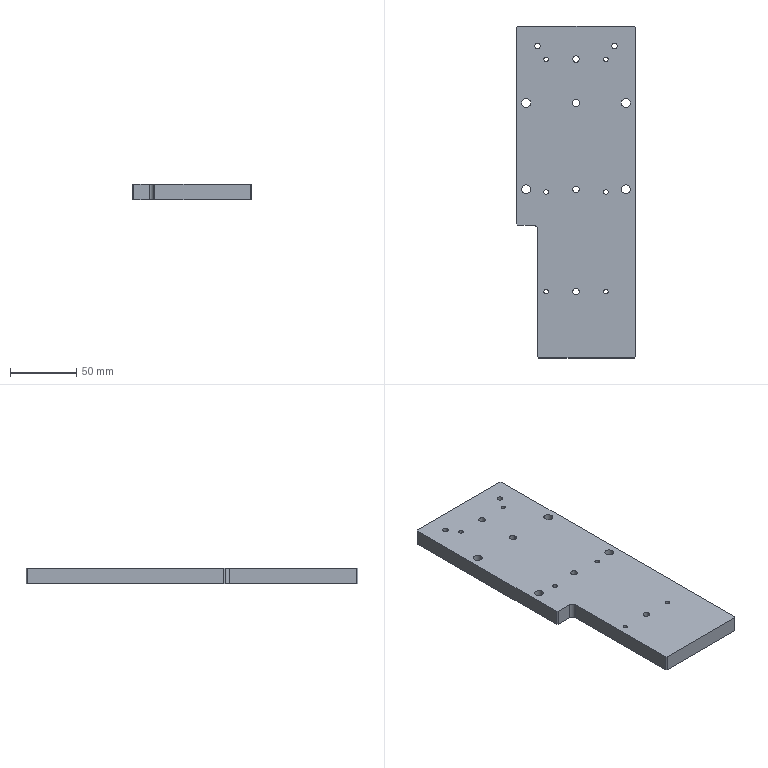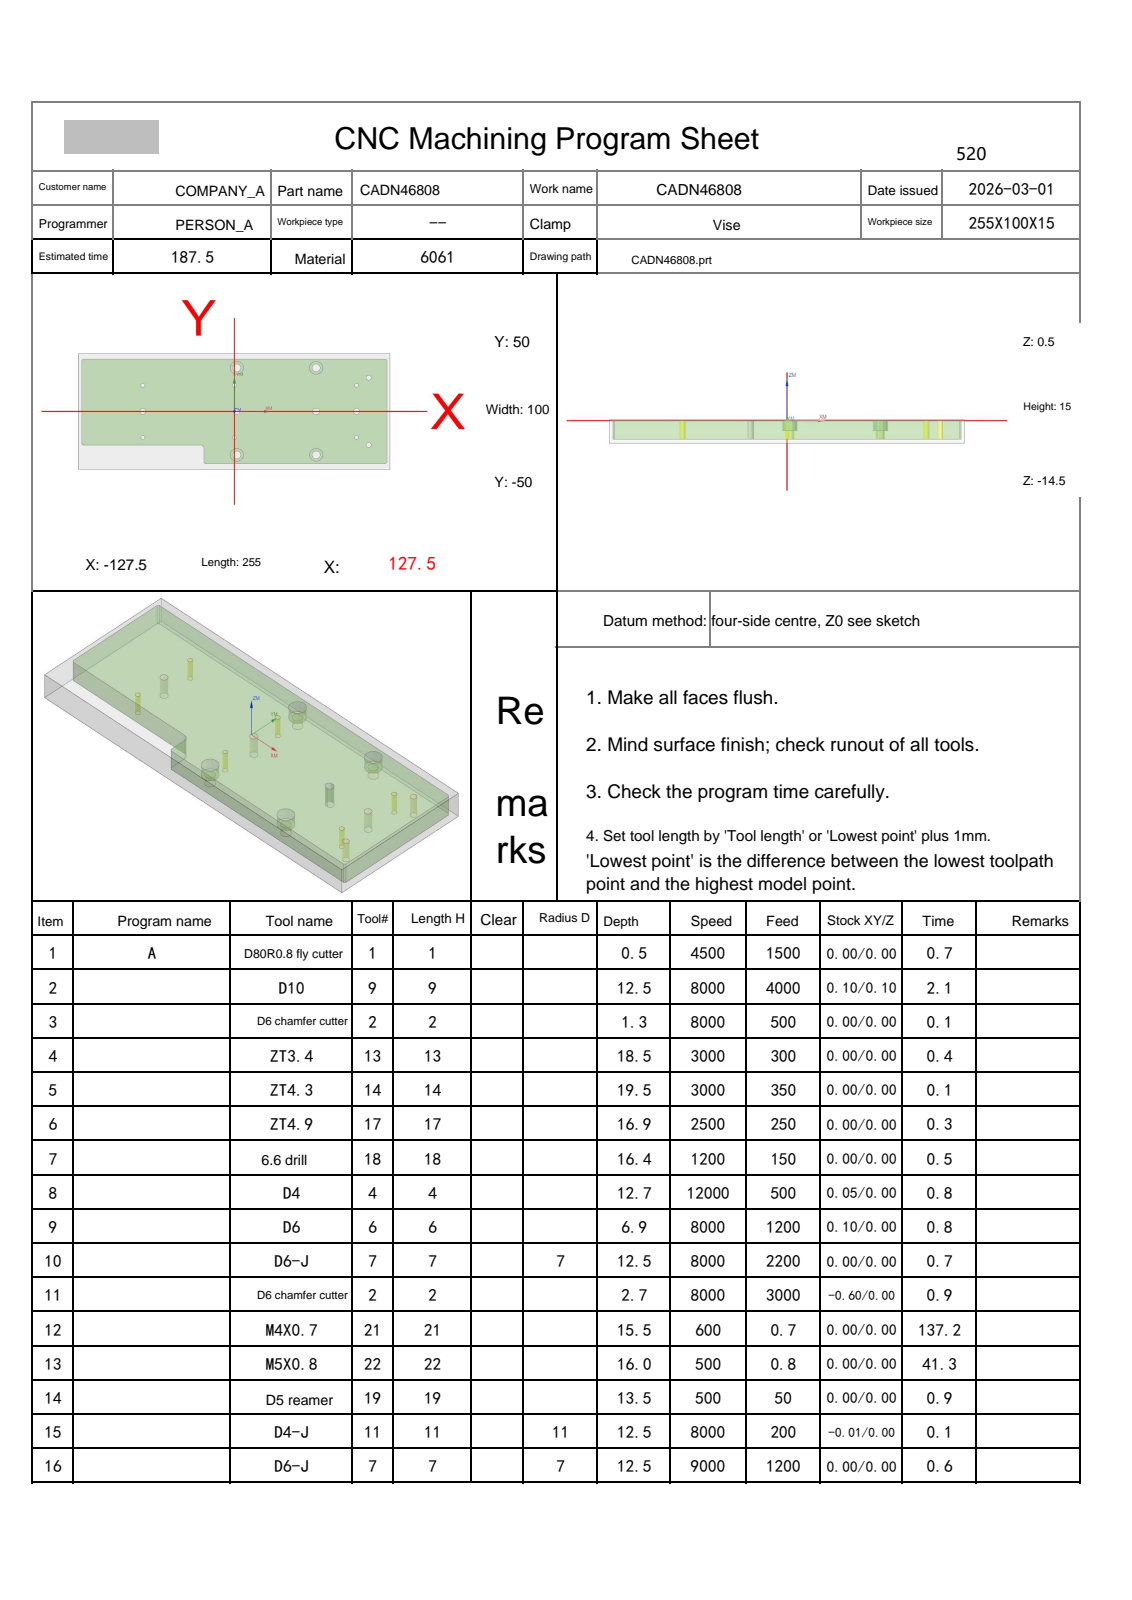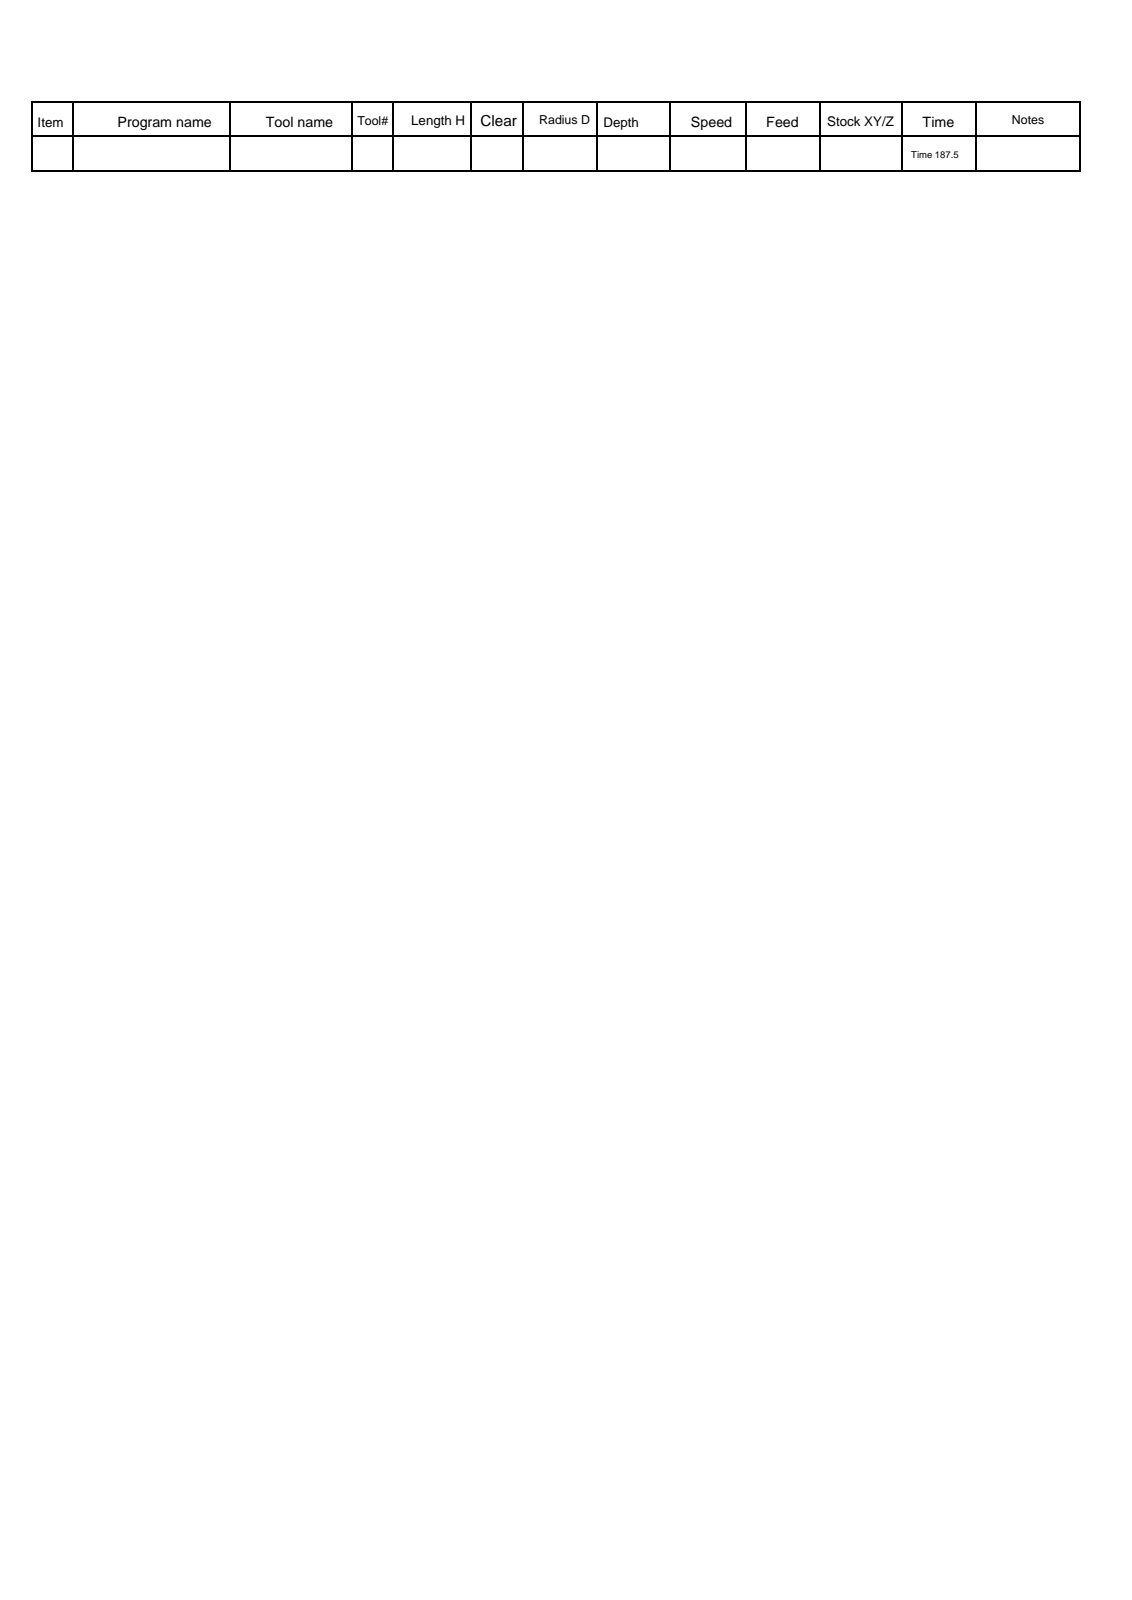NC program | NX | posted by the shop | part box 90 x 250 x 12 mm
Lines 1 to 1513 of 3445, first 1227 of 1511 lines:
%
O0001
(Machine time: 358.05 MIN)
(===Total Tool:14===)
(T1=D80R0.8 fly cutter D=80.  R=0.8  D-  H01 Z=0.    )
(T9=D10     D=10.  R=0.   D-  H09 Z=-12.  )
(T2=D6 chamfer cutter   D=6.   R=0.   D-  H02 Z=-2.2  )
(T13=ZT3.4  D=3.4  DR_a=118 D-  H13 Z=-18.  )
(T14=ZT4.3  D=4.3  DR_a=118 D-  H14 Z=-19.  )
(T17=ZT4.9  D=4.9  DR_a=120 D-  H17 Z=-16.41)
(T18=6.6 drill  D=6.6  DR_a=120 D-  H18 Z=-15.91)
(T4=D4      D=4.   R=0.   D-  H04 Z=-12.2 )
(T6=D6      D=6.   R=0.   D-  H06 Z=-6.4  )
(T7=D6-J    D=6.   R=0.   D7  H07 Z=-12.  )
(T21=M4X0.7 D=3.3  DR_a=180 D-  H21 Z=-15.  )
(T22=M5X0.8 D=4.2  DR_a=180 D-  H22 Z=-15.5 )
(T19=D5 reamer   D=5.   DR_a=180 D-  H19 Z=-13.  )
(T11=D4-J   D=4.   R=0.   D11 H11 Z=-12.  )
G80 G90 G17 G49 G40
G91 G28 Z0
M01
N1 T01 M06
(D80R0.8 fly cutter  D=80. R=0.8 H=01 ce=0.00 di=0.00)
G00 G90 G54 X-170. Y42.5 M03 S4500
G43 H01 Z50.
M08
Z2.
G01 Z0.0 F1500.
X-165.
X165.
Y0.0
X-165.
Y-42.5
X165.
X170.
Z2.
G00 Z50.
G91 G28 Z0.0
M05
M09
G91 G28 Z0.0
M01
N2 T09 M06
(D10  D=10. R=0. H=09 ce=0.10 di=0.10)
G00 G90 G54 X-125.158 Y61.447 M03 S8000
G43 H09 Z50.
M08
Z-10.
G01 X-125.141 Y61.348 Z-10.625 F4000.
X-125.125 Y61.25 Z-10.872
X-125.109 Y61.151 Z-11.054
X-125.092 Y61.052 Z-11.2
X-125.076 Y60.954 Z-11.323
X-125.06 Y60.855 Z-11.428
X-125.043 Y60.756 Z-11.52
X-125.027 Y60.658 Z-11.6
X-125.011 Y60.559 Z-11.67
X-124.994 Y60.46 Z-11.732
X-124.978 Y60.362 Z-11.786
X-124.962 Y60.263 Z-11.833
X-124.945 Y60.164 Z-11.874
X-124.929 Y60.066 Z-11.908
X-124.913 Y59.967 Z-11.936
X-124.896 Y59.868 Z-11.96
X-124.88 Y59.77 Z-11.977
X-124.864 Y59.671 Z-11.99
X-124.847 Y59.573 Z-11.997
X-124.831 Y59.474 Z-12.
X-124.487 Y57.397
G03 X-124.17 Y57.008 I.503 J.086
X-120.255 Y56.356 I4.038 J12.171
X-111.283 Y56.191 I8.972 J243.457
X-109.151 Y56.2 I0.0 J243.623
G01 X125.648 Y56.182
G02 X132.353 Y51.481 I-.009 J-7.145
X133.525 Y45.381 I-18.068 J-6.633
X133.718 Y35.276 I-263.984 J-10.105
X133.699 Y32.104 I-264.177 J0.0
G01 X133.679 Y-48.196
G02 X129.116 Y-54.791 I-7.099 J.036
X123.108 Y-56.009 I-6.605 J17.156
X113.899 Y-56.213 I-9.209 J207.731
X111.431 Y-56.199 I0.0 J207.935
G01 X-125.589 Y-56.184
X-125.654 Y-56.185
G02 X-132.289 Y-51.621 I0.0 J7.105
X-133.519 Y-45.454 I17.459 J6.69
X-133.712 Y-36.317 I217.075 J9.137
X-133.699 Y-33.937 I217.267 J0.0
G01 X-133.675 Y48.283
G02 X-129.102 Y54.798 I7.095 J-.117
X-124.661 Y55.615 I4.441 J-11.659
X-124.243 Y55.608 I0.0 J-12.476
G03 X-107.231 Y55.401 I18.077 J785.537
G01 X123.788 Y55.382
G02 X130.819 Y50.947 I-.125 J-7.989
X132.545 Y44.658 I-15.2 J-7.553
X132.897 Y36.148 I-102.586 J-8.509
X132.89 Y34.908 I-102.938 J0.0
G01 X132.878 Y-46.347
G02 X128.402 Y-53.339 I-8.005 J.196
X122.108 Y-55.05 I-7.546 J15.331
X113.513 Y-55.399 I-8.594 J105.535
X112.198 Y-55.391 I0.0 J105.885
G01 X-123.847 Y-55.378
G02 X-130.812 Y-50.953 I.187 J7.987
X-132.534 Y-44.747 I15.044 J7.517
X-132.9 Y-36.07 I102.672 J8.678
X-132.891 Y-34.678 I103.038 J0.0
G01 X-132.878 Y46.347
G02 X-127.751 Y53.506 I7.741 J-.128
X-121.795 Y54.573 I6.129 J-17.049
X-113.953 Y54.638 I7.842 J-472.
X-108.11 Y54.602 I0.0 J-472.066
G01 X122.028 Y54.58
G02 X129.881 Y49.564 I-.191 J-8.954
X131.724 Y42.728 I-16.901 J-8.222
X132.097 Y33.636 I-110.49 J-9.092
X132.09 Y32.339 I-110.863 J0.0
G01 X132.075 Y-44.601
G02 X127.083 Y-52.368 I-8.949 J.264
X120.403 Y-54.203 I-8.157 J16.616
X111.152 Y-54.599 I-9.251 J107.876
X109.695 Y-54.589 I0.0 J108.272
G01 X-121.965 Y-54.581
G02 X-129.839 Y-49.637 I.129 J8.948
X-131.723 Y-42.73 I16.736 J8.274
X-132.099 Y-33.56 I111.633 J9.171
X-132.09 Y-32.181 I112.009 J0.0
G01 X-132.081 Y44.439
G02 X-126.86 Y52.213 I8.466 J-.046
X-120.33 Y53.637 I7.215 J-17.401
X-112.344 Y53.823 I7.986 J-171.457
X-109.789 Y53.804 I0.0 J-171.642
G01 X120.268 Y53.779
G02 X128.972 Y48.325 I-.054 J-9.759
X130.894 Y41.182 I-18.023 J-8.678
X131.285 Y32.798 I-89.73 J-8.384
X131.28 Y31.835 I-90.121 J0.0
G01 X131.276 Y-42.785
G02 X125.794 Y-51.483 I-9.715 J.047
X118.801 Y-53.379 I-8.62 J17.949
X108.985 Y-53.801 I-9.816 J114.068
X107.373 Y-53.789 I0.0 J114.489
G01 X-120.287 Y-53.776
G02 X-129.121 Y-48.018 I.09 J9.793
X-130.904 Y-41.081 I18.797 J8.529
X-131.294 Y-31.667 I113.427 J9.414
X-131.287 Y-30.452 I113.817 J0.0
G01 X-131.275 Y42.808
Y42.811
G02 X-126.128 Y50.963 I9.029 J0.0
X-119.506 Y52.693 I7.884 J-16.63
X-111.144 Y53.008 I8.362 J-110.839
X-109.595 Y52.998 I0.0 J-111.154
G01 X118.545 Y52.981
X118.682 Y52.982
G02 X125.84 Y50.186 I0.0 J-10.562
G01 X126.615 Y49.372
G02 X129.219 Y46.866 I-5.969 J-8.805
X130.1 Y44.011 I-4.262 J-2.88
G03 X130.338 Y37.709 I135.671 J1.964
G02 X130.511 Y23.708 I-564.408 J-14.002
X130.498 Y19.791 I-564.581 J0.0
G01 X130.476 Y-41.069
G02 X130.1 Y-44.015 I-15.522 J.487
X128.388 Y-47.893 I-5.645 J.175
X121.214 Y-51.9 I-10.145 J9.738
X112.565 Y-52.883 I-9.072 J41.292
X101.253 Y-53.001 I-11.313 J540.846
X99.287 Y-52.998 I0.0 J540.964
G01 X-118.613 Y-52.975
X-118.717 Y-52.976
G02 X-126.168 Y-49.851 I0.0 J10.446
X-129.498 Y-43.2 I10.497 J9.414
X-130.406 Y-34.301 I45.044 J9.093
X-130.503 Y-22.532 I709.373 J11.77
X-130.498 Y-19.742 I709.47 J0.0
G01 X-130.477 Y41.038
G02 X-130.1 Y44.015 I20.16 J-1.041
X-128.283 Y47.946 I5.53 J-.17
X-123.993 Y50.623 I7.387 J-7.061
X-116.302 Y52.001 I8.574 J-25.718
X-106.011 Y52.215 I10.291 J-247.077
X-103.266 Y52.2 I0.0 J-247.291
G01 X116.954 Y52.18
X117.046
G02 X123.911 Y50.124 I0.0 J-12.489
G01 X125.329 Y49.928
G02 X126.672 Y49.334 I-9.033 J-22.267
G03 X125.329 Y49.928 I-10.376 J-21.674
G02 X121.666 Y50.698 I1.686 J17.109
G03 X114.654 Y51.504 I-7.012 J-30.093
G01 X114.448
G03 X105.805 Y51.562 I-8.644 J-639.404
X104.209 Y51.56 I0.0 J-639.462
G01 X-109.851 Y51.536
G03 X-110.63 Y51.541 I-.779 J-68.539
X-119.426 Y50.974 I0.0 J-68.544
X-123.087 Y50.1 I4.092 J-25.239
X-123.63 Y50.12 I-.542 J-7.145
X-125.563 Y49.854 I0.0 J-7.166
G01 X-126.66 Y49.351
X-125.563 Y49.854
X-124.821 Y50.034
G02 X-123.493 Y50.106 I1.328 J-12.134
X-123.087 Y50.1 I0.0 J-12.206
G03 X-117.888 Y50.386 I-.022 J47.735
G02 X-105.511 Y50.769 I12.377 J-199.641
X-103.177 Y50.756 I0.0 J-200.024
G01 X111.523 Y50.737
G02 X112.333 Y50.744 I.809 J-46.827
X119.652 Y50.169 I0.0 J-46.834
G01 X120.018 Y50.1
X123.998
X-124.061
G03 X-127.621 Y48.592 I.204 J-5.438
X-129.2 Y46.893 I9.138 J-10.075
X-130.1 Y43.923 I4.451 J-2.97
G01 Y43.906
Y-28.038
G02 X-129.702 Y-35.726 I-147.609 J-11.494
G03 X-128.536 Y-43.781 I33.867 J.789
X-124.572 Y-49.841 I11.22 J3.013
X-118.695 Y-52.007 I6.982 J9.888
X-111.231 Y-52.363 I7.464 J77.978
X-109.827 Y-52.351 I0.0 J78.335
G01 X107.273 Y-52.335
G03 X108.249 Y-52.341 I.977 J83.987
X117.971 Y-51.776 I0.0 J83.993
X123.877 Y-50.107 I-2.72 J20.908
X127.621 Y-48.592 I-.033 J5.464
X129.2 Y-46.892 I-11.663 J12.422
G02 X127.621 Y-48.592 I-10.674 J8.336
X123.793 Y-50.122 I-3.828 J4.021
X123.43 Y-50.11 I0.0 J5.552
G01 X117.478 Y-50.983
G02 X106.712 Y-51.537 I-10.766 J104.313
X105.897 Y-51.534 I0.0 J104.867
G01 X-111.443
G02 X-112.157 Y-51.54 I-.714 J44.451
X-118.698 Y-51.056 I0.0 J44.456
X-126.998 Y-44.388 I1.814 J10.756
X-128.698 Y-37.01 I22.356 J9.038
X-129.095 Y-31.098 I548.53 J39.845
G01 X-129.496 Y-30.406
G02 X-130.076 Y-28.23 I4.84 J2.454
G03 X-129.096 Y-31.038 I5.199 J.239
G02 X-128.366 Y-34.531 I-12.801 J-4.499
G03 X-127.217 Y-41.366 I44.929 J4.034
X-123.445 Y-47.662 I12.084 J2.963
X-117.035 Y-50.379 I8.114 J10.225
X-109.247 Y-50.901 I7.788 J57.793
X-108.419 Y-50.895 I0.0 J58.316
G01 X105.401 Y-50.892
G03 X106.334 Y-50.897 I.932 J104.039
X117.379 Y-50.309 I0.0 J104.043
G01 X118.951 Y-50.1
X123.671
X-107.582 Y-50.097
G02 X-108.465 Y-50.103 I-.883 J57.401
X-116.118 Y-49.591 I0.0 J57.408
X-122.714 Y-46.577 I1.589 J12.202
X-126.399 Y-40.111 I9.76 J9.845
X-127.68 Y-33.679 I70.118 J17.316
G03 X-128.14 Y-32.072 I-5.489 J-.701
G01 X-129.096 Y-31.038
G02 X-127.918 Y-32.359 I-27.507 J-25.723
X-126.792 Y-35.753 I-11.626 J-5.739
G03 X-124.972 Y-41.778 I30.45 J5.914
X-116.844 Y-48.473 I10.835 J4.873
X-109.315 Y-49.379 I7.791 J32.981
X-98.956 Y-49.479 I10.359 J540.85
X-97.316 Y-49.476 I0.0 J540.949
G01 X-26.456
X-25.32 Y-49.926
X-24.002 Y-50.1
X-25.32 Y-49.926
G03 X-29.695 Y-48.872 I-4.651 J-9.695
X-38.394 Y-48.664 I-8.699 J-182.449
X-40.57 Y-48.677 I0.0 J-182.657
G01 X-104.948 Y-48.654
G02 X-105.805 Y-48.66 I-.856 J61.413
X-114.043 Y-48.105 I0.0 J61.419
X-120.626 Y-45.369 I1.815 J13.655
X-124.817 Y-39.084 I9.226 J10.691
G01 X-126.476 Y-34.003
G03 X-126.899 Y-33.149 I-3.394 J-1.148
G02 X-128.116 Y-32.096 I4.596 J6.545
G03 X-126.775 Y-33.25 I6.473 J6.166
G02 X-125.391 Y-35.831 I-6.932 J-5.38
G03 X-123.052 Y-41.105 I32.848 J11.413
X-115.195 Y-46.923 I10.924 J6.539
X-107.435 Y-47.919 I8.207 J33.22
X-97.449 Y-48.038 I9.987 J418.237
X-95.997 Y-48.035 I0.0 J418.356
G01 X-35.499 Y-48.061
G02 X-34.723 Y-48.055 I.777 J-48.885
X-28.37 Y-48.469 I0.0 J-48.891
X-27.493 Y-48.693 I-1.559 J-7.951
G01 X-26.55 Y-49.417
G03 X-28.455 Y-48.183 I-4.66 J-5.107
X-33.158 Y-47.424 I-5.177 J-17.137
X-43.01 Y-47.223 I-9.852 J-241.104
X-45.528 Y-47.236 I0.0 J-241.306
G01 X-102.708 Y-47.21
G02 X-103.459 Y-47.214 I-.751 J64.868
X-112.042 Y-46.644 I0.0 J64.872
X-119.146 Y-43.739 I1.918 J14.829
X-123.329 Y-38.198 I10.308 J12.129
G03 X-125.375 Y-34.186 I-39.67 J-17.707
X-125.778 Y-33.736 I-1.507 J-.946
G02 X-126.867 Y-33.173 I.914 J3.103
G03 X-125.633 Y-33.804 I2.442 J3.255
G02 X-123.924 Y-35.976 I-4.861 J-5.585
G03 X-120.932 Y-40.698 I33.01 J17.605
X-112.702 Y-45.637 I11.094 J9.161
X-104.041 Y-46.516 I8.742 J42.995
X-94.093 Y-46.595 I9.948 J627.526
G01 X-93.642
X-39.179 Y-46.622
G02 X-38.433 Y-46.617 I.746 J-61.427
X-30.881 Y-47.083 I0.0 J-61.431
X-28.36 Y-47.81 I-.809 J-7.548
G01 X-27.608 Y-48.605
G03 X-29.105 Y-47.257 I-4.624 J-3.631
X-33.248 Y-46.194 I-5.094 J-11.257
X-42.27 Y-45.797 I-9.022 J-102.322
X-43.625 Y-45.806 I0.0 J-102.719
G01 X-100.848 Y-45.764
G02 X-101.511 Y-45.768 I-.662 J64.43
X-110.419 Y-45.149 I0.0 J64.433
X-118.072 Y-41.919 I2.152 J15.777
X-122.182 Y-37.079 I14.004 J16.059
G03 X-124.537 Y-34.083 I-12.61 J-7.489
X-125.32 Y-33.926 I-.864 J-2.273
G01 X-125.763 Y-33.743
G03 X-124.569 Y-34.036 I1.357 J2.946
G02 X-122.429 Y-35.965 I-3.339 J-5.856
G03 X-118.715 Y-40.263 I32.322 J24.17
X-110.256 Y-44.341 I11.188 J12.397
X-101.075 Y-45.101 I9.182 J55.048
G01 X-100.859
X-91.179 Y-45.155
X-42.531 Y-45.177
G02 X-41.583 Y-45.171 I.948 J-75.978
X-32.992 Y-45.658 I0.0 J-75.984
X-29.319 Y-46.724 I-1.044 J-10.457
G03 X-28.462 Y-47.702 I7.628 J5.83
G02 X-29.438 Y-46.558 I6.867 J6.85
G03 X-32.505 Y-45.208 I-4.287 J-5.578
X-39.978 Y-44.458 I-7.709 J-39.258
X-51.174 Y-44.355 I-11.196 J-608.546
G01 X-51.929 Y-44.356
X-98.528 Y-44.326
G02 X-99.284 Y-44.33 I-.755 J70.472
X-108.66 Y-43.703 I0.0 J70.476
X-119.757 Y-37.686 I2.384 J17.638
G03 X-122.897 Y-34.49 I-22.64 J-19.098
X-123.836 Y-34.089 I-.94 J-.9
G01 X-124.002 Y-34.1
X-124.715 Y-34.006
G03 X-123.434 Y-34.109 I1.475 J10.344
G02 X-121.044 Y-35.669 I-2.29 J-6.116
G03 X-116.773 Y-39.483 I38.096 J38.367
X-107.791 Y-43.043 I11.559 J16.054
X-98.159 Y-43.683 I9.632 J72.154
X-97.58 Y-43.68 I0.0 J72.794
G01 X-87.34 Y-43.716
X-45.01 Y-43.737
G02 X-44.05 Y-43.731 I.961 J-85.296
X-34.803 Y-44.234 I0.0 J-85.302
X-30.319 Y-45.509 I-1.31 J-13.134
X-29.657 Y-46.079 I-.498 J-1.247
G01 X-29.256 Y-46.772
G03 X-29.946 Y-45.604 I-7.483 J-3.637
X-32.968 Y-44.04 I-4.549 J-5.085
X-40.283 Y-43.085 I-7.957 J-32.453
X-51.884 Y-42.904 I-11.601 J-371.949
X-54.806 Y-42.915 I0.0 J-372.13
G01 X-96.466 Y-42.886
G02 X-97.185 Y-42.89 I-.718 J77.858
X-106.841 Y-42.289 I0.0 J77.861
X-118.206 Y-37.029 I2.733 J20.814
G03 X-121.705 Y-34.32 I-17.187 J-18.584
G01 X-122.221 Y-34.1
X-123.581
G02 X-122.961 Y-34.078 I.62 J-8.938
X-121.854 Y-34.147 I0.0 J-8.96
X-118.866 Y-35.839 I-3.316 J-9.337
G03 X-113.29 Y-39.494 I22.228 J27.832
X-104.202 Y-41.861 I11.073 J23.891
X-93.972 Y-42.271 I10.231 J127.253
X-92.694 Y-42.265 I0.0 J127.664
G01 X-46.853 Y-42.299
G02 X-45.959 Y-42.295 I.895 J-88.655
X-36.167 Y-42.837 I0.0 J-88.659
X-31.107 Y-44.288 I-1.505 J-14.794
X-29.925 Y-45.257 I-1.351 J-2.854
G01 X-29.677 Y-46.017
G03 X-30.293 Y-44.634 I-3.43 J-.699
X-33.557 Y-42.803 I-5.064 J-5.203
X-41.197 Y-41.687 I-8.499 J-31.485
X-52.375 Y-41.469 I-11.178 J-286.059
X-54.329 Y-41.475 I0.0 J-286.278
G01 X-94.688 Y-41.445
G02 X-95.452 Y-41.449 I-.764 J80.238
X-105.621 Y-40.802 I0.0 J80.242
X-116.731 Y-36.282 I3.712 J25.037
G03 X-120.35 Y-34.119 I-13.265 J-18.091
G01 X-122.212 Y-34.1
G02 X-121.831 Y-34.098 I.381 J-44.546
X-120.085 Y-34.132 I0.0 J-44.548
X-116.915 Y-35.559 I-3.127 J-11.182
G03 X-110.243 Y-38.87 I19.711 J31.34
X-100.745 Y-40.578 I10.996 J33.882
X-89.198 Y-40.848 I11.547 J246.81
X-86.509 Y-40.833 I0.0 J247.08
G01 X-49.089 Y-40.857
G02 X-48.105 Y-40.852 I.985 J-100.333
X-37.656 Y-41.397 I0.0 J-100.338
X-31.869 Y-42.982 I-1.649 J-17.375
X-30.069 Y-44.492 I-1.934 J-4.135
G01 X-29.963 Y-45.139
G03 X-31.064 Y-43.107 I-2.563 J-.074
X-35.671 Y-41.107 I-6.662 J-9.037
X-44.631 Y-40.167 I-9.525 J-47.665
X-56.596 Y-40.031 I-11.965 J-524.426
X-58.649 Y-40.035 I0.0 J-524.562
G01 X-92.708 Y-40.007
G02 X-93.537 Y-40.011 I-.829 J88.735
X-104.123 Y-39.377 I0.0 J88.739
X-115.045 Y-35.621 I4.412 J30.583
G03 X-118.243 Y-34.1 I-11.321 J-19.686
G01 X-120.403
G02 X-119.45 Y-34.078 I.953 J-20.374
X-117.651 Y-34.157 I0.0 J-20.396
X-114.579 Y-35.28 I-4.054 J-15.855
G03 X-105.622 Y-38.369 I16.997 J34.749
X-94.877 Y-39.316 I10.937 J62.686
X-84.096 Y-39.399 I10.782 J698.601
X-81.598 Y-39.395 I0.0 J698.684
G01 X-50.137 Y-39.423
G02 X-49.422 Y-39.421 I.715 J-99.596
X-38.627 Y-40.007 I0.0 J-99.599
X-32.54 Y-41.658 I-1.983 J-19.367
X-30.137 Y-43.697 I-2.224 J-5.055
G01 X-30.041 Y-44.556
Y-44.539
G03 X-30.222 Y-43.34 I-4.075 J0.0
X-32.707 Y-41.062 I-4.758 J-2.696
X-39.038 Y-39.267 I-8.418 J-17.636
X-49.907 Y-38.636 I-10.869 J-93.311
G01 X-50.219 Y-38.637
X-60.408 Y-38.595
X-91.568 Y-38.561
G02 X-92.197 Y-38.564 I-.628 J90.084
X-103.141 Y-37.896 I0.0 J90.087
X-113.216 Y-34.955 I5.947 J39.101
G03 X-115.484 Y-34.1 I-29.245 J-74.121
G01 X-118.124
G02 X-116.943 Y-34.082 I1.181 J-39.028
X-114.819 Y-34.14 I0.0 J-39.046
X-110.467 Y-35.393 I-6.293 J-30.034
G03 X-96.796 Y-37.759 I14.988 J45.929
X-83.318 Y-37.973 I13.478 J424.552
X-79.358 Y-37.954 I0.0 J424.766
G01 X-51.342 Y-37.988
G02 X-50.754 Y-37.986 I.588 J-100.964
X-39.516 Y-38.613 I0.0 J-100.966
X-32.946 Y-40.415 I-2.194 J-20.879
X-30.18 Y-42.81 I-2.55 J-5.739
X-30.08 Y-43.534 I-2.558 J-.724
X-30.1 Y-43.862 I-2.659 J0.0
G03 X-30.076 Y-43.469 I-3.203 J.393
X-30.274 Y-42.357 I-3.227 J0.0
X-32.94 Y-39.878 I-5.312 J-3.04
X-39.611 Y-37.908 I-9.016 J-18.254
X-50.919 Y-37.207 I-11.308 J-90.848
G01 X-51.029
X-61.848 Y-37.155
X-89.588 Y-37.125
G02 X-90.363 Y-37.128 I-.775 J101.669
X-101.963 Y-36.465 I0.0 J101.672
X-111.57 Y-34.178 I8.745 J58.075
G01 X-111.883 Y-34.1
X-115.323
G02 X-113.678 Y-34.077 I1.645 J-59.152
X-110.703 Y-34.152 I0.0 J-59.175
X-104.836 Y-35.305 I-24.317 J-139.213
G03 X-91.701 Y-36.441 I13.343 J77.751
X-80.947 Y-36.521 I10.754 J728.148
X-77.941 Y-36.514 I0.0 J728.227
G01 X-53.178 Y-36.544
G02 X-52.491 Y-36.542 I.686 J-111.331
X-40.617 Y-37.177 I0.0 J-111.333
X-33.529 Y-39.042 I-2.405 J-23.54
X-30.339 Y-41.612 I-2.992 J-6.978
X-30.1 Y-42.143 I-2.84 J-1.599
G01 Y-43.023
G03 X-30.076 Y-42.598 I-3.798 J.424
X-30.252 Y-41.453 I-3.822 J0.0
X-32.915 Y-38.804 I-5.538 J-2.905
X-39.481 Y-36.653 I-9.347 J-17.434
X-50.658 Y-35.801 I-11.564 J-77.938
G01 X-60.409 Y-35.715
X-88.788 Y-35.678
G02 X-89.35 Y-35.68 I-.562 J102.536
X-102.432 Y-34.842 I0.0 J102.537
G01 X-106.585 Y-34.1
X-111.385
G02 X-108.711 Y-34.076 I2.674 J-150.193
X-103.902 Y-34.153 I0.0 J-150.217
G03 X-86.468 Y-35.061 I17.435 J166.899
X-85.469 Y-35.058 I0.0 J167.808
G01 X-54.142 Y-35.109
G02 X-53.546 Y-35.108 I.596 J-110.469
X-41.196 Y-35.8 I0.0 J-110.471
X-33.717 Y-37.83 I-2.619 J-24.445
X-30.334 Y-40.624 I-3.236 J-7.364
X-30.1 Y-41.168 I-2.458 J-1.38
G01 Y-42.128
G03 X-30.08 Y-41.67 I-5.337 J.458
X-30.18 Y-40.639 I-5.357 J0.0
X-32.492 Y-37.967 I-5.287 J-2.237
X-38.926 Y-35.492 I-9.576 J-15.297
X-49.515 Y-34.432 I-11.662 J-63.044
X-63.758 Y-34.264 I-14.243 J-605.708
X-67.369 Y-34.275 I0.0 J-605.876
G01 X-88.049 Y-34.23
G03 X-100.22 Y-34.077 I-12.171 J-482.238
X-104.96 Y-34.1 I0.0 J-482.392
G01 X-45.452 Y-34.12
G02 X-35.5 Y-35.901 I-.871 J-33.565
X-30.86 Y-38.844 I-3.536 J-10.705
X-30.1 Y-40.12 I-2.641 J-2.437
G01 Y-41.08
G03 X-30.075 Y-40.611 I-4.413 J.469
X-30.239 Y-39.416 I-4.438 J0.0
X-32.882 Y-36.578 I-5.911 J-2.856
X-39.593 Y-34.1 I-10.061 J-16.919
G01 X-46.153
X-38.326 Y-34.123
G02 X-31.145 Y-37.435 I-1.233 J-12.117
X-30.1 Y-39.044 I-2.856 J-2.997
G01 Y-40.004
G03 X-30.077 Y-39.54 I-4.601 J.464
X-30.234 Y-38.343 I-4.625 J0.0
X-32.891 Y-35.45 I-5.951 J-2.799
X-35.786 Y-34.1 I-6.516 J-10.194
G01 X-38.746
G02 X-37.44 Y-34.079 I1.305 J-39.724
X-35.147 Y-34.145 I0.0 J-39.745
X-30.269 Y-37.534 I-1.436 J-7.27
G01 X-30.1 Y-37.972
Y-38.932
G03 X-30.076 Y-38.463 I-4.52 J.47
X-30.241 Y-37.246 I-4.545 J0.0
X-33.746 Y-34.1 I-5.475 J-2.573
G01 X-35.586
G02 X-34.864 Y-34.089 I.722 J-23.292
X-33.375 Y-34.136 I0.0 J-23.304
X-30.108 Y-36.892 I-1.197 J-4.733
G01 X-30.1 Y-37.818
G03 X-30.077 Y-37.387 I-3.998 J.431
X-30.241 Y-36.25 I-4.021 J0.0
X-32.468 Y-34.1 I-3.545 J-1.444
G01 X-33.668
G02 X-33.138 Y-34.08 I.53 J-7.121
X-32.1 Y-34.156 I0.0 J-7.14
X-30.1 Y-36.063 I-.919 J-2.967
G01 Y-36.783
G03 X-30.075 Y-36.418 I-2.684 J.365
X-30.364 Y-35.201 I-2.708 J0.0
X-31.642 Y-34.1 I-1.975 J-1.
G01 X-32.442
G02 X-32.071 Y-34.08 I.371 J-3.372
X-31.275 Y-34.174 I0.0 J-3.392
X-30.1 Y-35.422 I-.722 J-1.858
G01 Y-36.062
G03 X-30.076 Y-35.739 I-2.156 J.323
X-30.325 Y-34.728 I-2.18 J0.0
X-31.371 Y-34.079 I-1.046 J-.52
X-31.591 Y-34.1 I0.0 J-1.168
G02 X-31.339 Y-34.075 I.252 J-1.273
X-30.1 Y-34.988 I0.0 J-1.298
G01 Y-35.388
G03 X-30.078 Y-35.159 I-1.17 J.229
X-30.659 Y-34.135 I-1.192 J0.0
G01 X-31.097 Y-34.1
X-30.907 Y-34.077
G02 X-30.098 Y-34.886 I0.0 J-.809
G01 X-30.1 Y-34.945
X-30.08 Y-34.781
G03 X-30.761 Y-34.1 I-.681 J0.0
G01 X-30.785
G03 X-31.202 Y-34.319 I.004 J-.512
G01 X-32.535 Y-36.264
X-32.6 Y-36.408
X-32.623 Y-36.565
X-32.62 Y-36.665 Z-11.997
X-32.617 Y-36.765 Z-11.99
X-32.614 Y-36.865 Z-11.977
X-32.611 Y-36.964 Z-11.96
X-32.609 Y-37.064 Z-11.936
X-32.606 Y-37.164 Z-11.908
X-32.603 Y-37.264 Z-11.874
X-32.6 Y-37.364 Z-11.833
X-32.597 Y-37.464 Z-11.786
X-32.594 Y-37.564 Z-11.732
X-32.591 Y-37.664 Z-11.67
X-32.588 Y-37.764 Z-11.6
X-32.585 Y-37.864 Z-11.52
X-32.582 Y-37.964 Z-11.428
X-32.579 Y-38.064 Z-11.323
X-32.576 Y-38.164 Z-11.2
X-32.573 Y-38.264 Z-11.054
X-32.571 Y-38.364 Z-10.872
X-32.568 Y-38.464 Z-10.625
X-32.565 Y-38.564 Z-10.
G00 Z50.
X132.716 Y45.55
Z-10.
G01 X132.708 Y45.45 Z-10.625
X132.701 Y45.35 Z-10.872
X132.693 Y45.251 Z-11.054
X132.686 Y45.151 Z-11.2
X132.678 Y45.051 Z-11.323
X132.671 Y44.951 Z-11.428
X132.663 Y44.852 Z-11.52
X132.655 Y44.752 Z-11.6
X132.648 Y44.652 Z-11.67
X132.64 Y44.553 Z-11.732
X132.633 Y44.453 Z-11.786
X132.625 Y44.353 Z-11.833
X132.618 Y44.253 Z-11.874
X132.61 Y44.154 Z-11.908
X132.602 Y44.054 Z-11.936
X132.595 Y43.954 Z-11.96
X132.587 Y43.855 Z-11.977
X132.58 Y43.755 Z-11.99
X132.572 Y43.655 Z-11.997
X132.565 Y43.555 Z-12.
G02 X132.061 Y43.089 I-.504 J.039
G01 X131.978 Y43.096
X130.688 Y43.31
X130.605 Y43.316
G03 X130.1 Y42.811 I0.0 J-.505
G01 Y-44.015
G03 X130.486 Y-44.506 I.507 J.001
G01 X132.475 Y-44.989
X132.572 Y-45.013 Z-11.997
X132.669 Y-45.037 Z-11.99
X132.766 Y-45.06 Z-11.977
X132.864 Y-45.084 Z-11.96
X132.961 Y-45.107 Z-11.936
X133.058 Y-45.131 Z-11.908
X133.155 Y-45.155 Z-11.874
X133.252 Y-45.178 Z-11.833
X133.349 Y-45.202 Z-11.786
X133.447 Y-45.226 Z-11.732
X133.544 Y-45.249 Z-11.67
X133.641 Y-45.273 Z-11.6
X133.738 Y-45.296 Z-11.52
X133.835 Y-45.32 Z-11.428
X133.932 Y-45.344 Z-11.323
X134.03 Y-45.367 Z-11.2
X134.127 Y-45.391 Z-11.054
X134.224 Y-45.415 Z-10.872
X134.321 Y-45.438 Z-10.625
X134.418 Y-45.462 Z-10.
G00 Z50.
G91 G28 Z0.0
M05
M09
G91 G28 Z0.0
M01
N3 T02 M06
(D6 chamfer cutter  D=6. R=0. H=02 ce=0.00 di=0.10)
G00 G90 G54 X67. Y-37.5 M03 S8000
G43 H02 Z50.
M08
G98 G81 X67. Y-37.5 Z-.8 R1. F500.
X110. Y-29.
X100. Y-22.5
Y0.0
Y22.5
X110. Y29.
X67. Y37.5
X2.
X0.0 Y22.5
X2. Y0.0
X0.0 Y-22.5
X2. Y-37.5
X-75. Y-22.5
Y0.0
Y22.5
G80
G00 Z50.
G00 G90 X66.5 Y0.0 M03 S8000
Z50.
G98 G81 X66.5 Y0.0 Z-.8 R1. F500.
G80
G00 Z50.
G91 G28 Z0.0
M05
M09
G91 G28 Z0.0
M01
N4 T13 M06
(ZT3.4 D=3.4 DR_a=118 H=13)
G00 G90 G54 X100. Y22.5 M03 S3000
G43 H13 Z50.
M08
G98 G83 X100. Y22.5 Z-18. R1. F300. Q2.
Y-22.5
X0.0
Y22.5
X-75.
Y-22.5
G80
G00 Z50.
G91 G28 Z0.0
M05
M09
G91 G28 Z0.0
M01
N5 T14 M06
(ZT4.3 D=4.3 DR_a=118 H=14)
G00 G90 G54 X110. Y29. M03 S3000
G43 H14 Z50.
M08
G98 G83 X110. Y29. Z-19. R1. F350. Q3.
Y-29.
G80
G00 Z50.
G91 G28 Z0.0
M05
M09
G91 G28 Z0.0
M01
N6 T17 M06
(ZT4.9 D=4.9 DR_a=120 H=17)
G00 G90 G54 X100. Y0.0 M03 S2500
G43 H17 Z50.
M08
G98 G83 X100. Y0.0 Z-16.415 R1. F250. Q2.
X2.
X-75.
G80
G00 Z50.
G00 G90 X66.5 Y0.0 M03 S2500
Z50.
G98 G83 X66.5 Y0.0 Z-16.415 R1. F250. Q2.
G80
G00 Z50.
G91 G28 Z0.0
M05
M09
G91 G28 Z0.0
M01
N7 T18 M06
(6.6 drill D=6.6 DR_a=120 H=18)
G00 G90 G54 X2. Y-37.5 M03 S1200
G43 H18 Z50.
M08
G98 G83 X2. Y-37.5 Z-15.905 R1. F150. Q2.
X67.
Y37.5
X2.
G80
G00 Z50.
G91 G28 Z0.0
M05
M09
G91 G28 Z0.0
M01
N8 T04 M06
(D4  D=4. R=0. H=04 ce=0.05 di=0.00)
G00 G90 G54 X67. Y-.45 M03 S12000
G43 H04 Z50.
M08
Z.5
G01 X67.5 Z.485 F500.
G03 X67.95 Y0.0 Z.463 I0.0 J.45
X67.785 Y.349 Z.45 I-.45 J0.0
X67.5 Y.45 Z.441 I-.285 J-.349
G01 X66.5 Z.41
G03 X66.05 Y0.0 Z.388 I0.0 J-.45
X66.5 Y-.45 Z.366 I.45 J0.0
G01 X67.5 Z.335
G03 X67.95 Y0.0 Z.313 I0.0 J.45
X67.785 Y.349 Z.301 I-.45 J0.0
X67.5 Y.45 Z.291 I-.285 J-.349
G01 X66.5 Z.26
G03 X66.05 Y0.0 Z.239 I0.0 J-.45
X66.5 Y-.45 Z.217 I.45 J0.0
G01 X67.5 Z.186
G03 X67.95 Y0.0 Z.164 I0.0 J.45
X67.785 Y.349 Z.151 I-.45 J0.0
X67.5 Y.45 Z.142 I-.285 J-.349
G01 X66.5 Z.111
G03 X66.05 Y0.0 Z.089 I0.0 J-.45
X66.5 Y-.45 Z.067 I.45 J0.0
G01 X67.5 Z.036
G03 X67.95 Y0.0 Z.014 I0.0 J.45
X67.785 Y.349 Z.002 I-.45 J0.0
X67.5 Y.45 Z-.007 I-.285 J-.349
G01 X66.5 Z-.038
G03 X66.05 Y0.0 Z-.06 I0.0 J-.45
X66.5 Y-.45 Z-.082 I.45 J0.0
G01 X67.5 Z-.113
G03 X67.95 Y0.0 Z-.135 I0.0 J.45
X67.785 Y.349 Z-.147 I-.45 J0.0
X67.5 Y.45 Z-.157 I-.285 J-.349
G01 X66.5 Z-.188
G03 X66.05 Y0.0 Z-.21 I0.0 J-.45
X66.5 Y-.45 Z-.232 I.45 J0.0
G01 X67.5 Z-.263
G03 X67.95 Y0.0 Z-.284 I0.0 J.45
X67.785 Y.349 Z-.297 I-.45 J0.0
X67.5 Y.45 Z-.306 I-.285 J-.349
G01 X66.5 Z-.337
G03 X66.05 Y0.0 Z-.359 I0.0 J-.45
X66.5 Y-.45 Z-.381 I.45 J0.0
G01 X67.5 Z-.412
G03 X67.95 Y0.0 Z-.434 I0.0 J.45
X67.785 Y.349 Z-.446 I-.45 J0.0
X67.5 Y.45 Z-.456 I-.285 J-.349
G01 X66.5 Z-.487
G03 X66.05 Y0.0 Z-.509 I0.0 J-.45
X66.5 Y-.45 Z-.53 I.45 J0.0
G01 X67.5 Z-.561
G03 X67.95 Y0.0 Z-.583 I0.0 J.45
X67.785 Y.349 Z-.596 I-.45 J0.0
X67.5 Y.45 Z-.605 I-.285 J-.349
G01 X66.5 Z-.636
G03 X66.05 Y0.0 Z-.658 I0.0 J-.45
X66.5 Y-.45 Z-.68 I.45 J0.0
G01 X67.5 Z-.711
G03 X67.95 Y0.0 Z-.733 I0.0 J.45
X67.785 Y.349 Z-.745 I-.45 J0.0
X67.5 Y.45 Z-.755 I-.285 J-.349
G01 X66.5 Z-.785
G03 X66.05 Y0.0 Z-.807 I0.0 J-.45
X66.5 Y-.45 Z-.829 I.45 J0.0
G01 X67.5 Z-.86
G03 X67.95 Y0.0 Z-.882 I0.0 J.45
X67.785 Y.349 Z-.894 I-.45 J0.0
X67.5 Y.45 Z-.904 I-.285 J-.349
G01 X66.5 Z-.935
G03 X66.05 Y0.0 Z-.957 I0.0 J-.45
X66.5 Y-.45 Z-.979 I.45 J0.0
G01 X67.5 Z-1.01
G03 X67.95 Y0.0 Z-1.031 I0.0 J.45
X67.785 Y.349 Z-1.044 I-.45 J0.0
X67.5 Y.45 Z-1.053 I-.285 J-.349
G01 X66.5 Z-1.084
G03 X66.05 Y0.0 Z-1.106 I0.0 J-.45
X66.5 Y-.45 Z-1.128 I.45 J0.0
G01 X67.5 Z-1.159
G03 X67.95 Y0.0 Z-1.181 I0.0 J.45
X67.785 Y.349 Z-1.193 I-.45 J0.0
X67.5 Y.45 Z-1.203 I-.285 J-.349
G01 X66.5 Z-1.234
G03 X66.05 Y0.0 Z-1.256 I0.0 J-.45
X66.5 Y-.45 Z-1.277 I.45 J0.0
G01 X67.5 Z-1.308
G03 X67.95 Y0.0 Z-1.33 I0.0 J.45
X67.785 Y.349 Z-1.343 I-.45 J0.0
X67.5 Y.45 Z-1.352 I-.285 J-.349
G01 X66.5 Z-1.383
G03 X66.05 Y0.0 Z-1.405 I0.0 J-.45
X66.5 Y-.45 Z-1.427 I.45 J0.0
G01 X67.5 Z-1.458
G03 X67.95 Y0.0 Z-1.48 I0.0 J.45
X67.785 Y.349 Z-1.492 I-.45 J0.0
X67.5 Y.45 Z-1.502 I-.285 J-.349
G01 X66.5 Z-1.533
G03 X66.05 Y0.0 Z-1.554 I0.0 J-.45
X66.5 Y-.45 Z-1.576 I.45 J0.0
G01 X67.5 Z-1.607
G03 X67.95 Y0.0 Z-1.629 I0.0 J.45
X67.785 Y.349 Z-1.641 I-.45 J0.0
X67.5 Y.45 Z-1.651 I-.285 J-.349
G01 X66.5 Z-1.682
G03 X66.05 Y0.0 Z-1.704 I0.0 J-.45
X66.5 Y-.45 Z-1.726 I.45 J0.0
G01 X67.5 Z-1.757
G03 X67.95 Y0.0 Z-1.779 I0.0 J.45
X67.785 Y.349 Z-1.791 I-.45 J0.0
X67.5 Y.45 Z-1.8 I-.285 J-.349
G01 X66.5 Z-1.831
G03 X66.05 Y0.0 Z-1.853 I0.0 J-.45
X66.5 Y-.45 Z-1.875 I.45 J0.0
G01 X67.5 Z-1.906
G03 X67.95 Y0.0 Z-1.928 I0.0 J.45
X67.785 Y.349 Z-1.94 I-.45 J0.0
X67.5 Y.45 Z-1.95 I-.285 J-.349
G01 X66.5 Z-1.981
G03 X66.05 Y0.0 Z-2.003 I0.0 J-.45
X66.5 Y-.45 Z-2.025 I.45 J0.0
G01 X67.5 Z-2.055
G03 X67.95 Y0.0 Z-2.077 I0.0 J.45
X67.785 Y.349 Z-2.09 I-.45 J0.0
X67.5 Y.45 Z-2.099 I-.285 J-.349
G01 X66.5 Z-2.13
G03 X66.05 Y0.0 Z-2.152 I0.0 J-.45
X66.5 Y-.45 Z-2.174 I.45 J0.0
G01 X67.5 Z-2.205
G03 X67.95 Y0.0 Z-2.227 I0.0 J.45
X67.785 Y.349 Z-2.239 I-.45 J0.0
X67.5 Y.45 Z-2.249 I-.285 J-.349
G01 X66.5 Z-2.28
G03 X66.05 Y0.0 Z-2.301 I0.0 J-.45
X66.5 Y-.45 Z-2.323 I.45 J0.0
G01 X67.5 Z-2.354
G03 X67.95 Y0.0 Z-2.376 I0.0 J.45
X67.785 Y.349 Z-2.389 I-.45 J0.0
X67.5 Y.45 Z-2.398 I-.285 J-.349
G01 X66.5 Z-2.429
G03 X66.05 Y0.0 Z-2.451 I0.0 J-.45
X66.5 Y-.45 Z-2.473 I.45 J0.0
G01 X67.5 Z-2.504
G03 X67.95 Y0.0 Z-2.526 I0.0 J.45
X67.785 Y.349 Z-2.538 I-.45 J0.0
X67.5 Y.45 Z-2.547 I-.285 J-.349
G01 X66.5 Z-2.578
G03 X66.05 Y0.0 Z-2.6 I0.0 J-.45
X66.5 Y-.45 Z-2.622 I.45 J0.0
G01 X67.5 Z-2.653
G03 X67.95 Y0.0 Z-2.675 I0.0 J.45
X67.785 Y.349 Z-2.687 I-.45 J0.0
X67.5 Y.45 Z-2.697 I-.285 J-.349
G01 X66.5 Z-2.728
G03 X66.05 Y0.0 Z-2.75 I0.0 J-.45
X66.5 Y-.45 Z-2.772 I.45 J0.0
G01 X67.5 Z-2.803
G03 X67.95 Y0.0 Z-2.824 I0.0 J.45
X67.785 Y.349 Z-2.837 I-.45 J0.0
X67.5 Y.45 Z-2.846 I-.285 J-.349
G01 X66.5 Z-2.877
G03 X66.05 Y0.0 Z-2.899 I0.0 J-.45
X66.5 Y-.45 Z-2.921 I.45 J0.0
G01 X67.5 Z-2.952
G03 X67.95 Y0.0 Z-2.974 I0.0 J.45
X67.785 Y.349 Z-2.986 I-.45 J0.0
X67.5 Y.45 Z-2.996 I-.285 J-.349
G01 X66.5 Z-3.027
G03 X66.05 Y0.0 Z-3.049 I0.0 J-.45
X66.5 Y-.45 Z-3.07 I.45 J0.0
G01 X67.5 Z-3.101
G03 X67.95 Y0.0 Z-3.123 I0.0 J.45
X67.785 Y.349 Z-3.136 I-.45 J0.0
X67.5 Y.45 Z-3.145 I-.285 J-.349
G01 X66.5 Z-3.176
G03 X66.05 Y0.0 Z-3.198 I0.0 J-.45
X66.5 Y-.45 Z-3.22 I.45 J0.0
G01 X67.5 Z-3.251
G03 X67.95 Y0.0 Z-3.273 I0.0 J.45
X67.785 Y.349 Z-3.285 I-.45 J0.0
X67.5 Y.45 Z-3.295 I-.285 J-.349
G01 X66.5 Z-3.325
G03 X66.05 Y0.0 Z-3.347 I0.0 J-.45
X66.5 Y-.45 Z-3.369 I.45 J0.0
G01 X67.5 Z-3.4
G03 X67.95 Y0.0 Z-3.422 I0.0 J.45
X67.785 Y.349 Z-3.434 I-.45 J0.0
X67.5 Y.45 Z-3.444 I-.285 J-.349
G01 X66.5 Z-3.475
G03 X66.05 Y0.0 Z-3.497 I0.0 J-.45
X66.5 Y-.45 Z-3.519 I.45 J0.0
G01 X67.5 Z-3.55
G03 X67.95 Y0.0 Z-3.571 I0.0 J.45
X67.785 Y.349 Z-3.584 I-.45 J0.0
X67.5 Y.45 Z-3.593 I-.285 J-.349
G01 X66.5 Z-3.624
G03 X66.05 Y0.0 Z-3.646 I0.0 J-.45
X66.5 Y-.45 Z-3.668 I.45 J0.0
G01 X67.5 Z-3.699
G03 X67.95 Y0.0 Z-3.721 I0.0 J.45
X67.785 Y.349 Z-3.733 I-.45 J0.0
X67.5 Y.45 Z-3.743 I-.285 J-.349
G01 X66.5 Z-3.774
G03 X66.05 Y0.0 Z-3.796 I0.0 J-.45
X66.5 Y-.45 Z-3.817 I.45 J0.0
G01 X67.5 Z-3.848
G03 X67.95 Y0.0 Z-3.87 I0.0 J.45
X67.785 Y.349 Z-3.883 I-.45 J0.0
X67.5 Y.45 Z-3.892 I-.285 J-.349
G01 X66.5 Z-3.923
G03 X66.05 Y0.0 Z-3.945 I0.0 J-.45
X66.5 Y-.45 Z-3.967 I.45 J0.0
G01 X67.5 Z-3.998
G03 X67.95 Y0.0 Z-4.02 I0.0 J.45
X67.785 Y.349 Z-4.032 I-.45 J0.0
X67.5 Y.45 Z-4.042 I-.285 J-.349
G01 X66.5 Z-4.073
G03 X66.05 Y0.0 Z-4.094 I0.0 J-.45
X66.5 Y-.45 Z-4.116 I.45 J0.0
G01 X67.5 Z-4.147
G03 X67.95 Y0.0 Z-4.169 I0.0 J.45
X67.785 Y.349 Z-4.181 I-.45 J0.0
X67.5 Y.45 Z-4.191 I-.285 J-.349
G01 X66.5 Z-4.222
G03 X66.05 Y0.0 Z-4.244 I0.0 J-.45
X66.5 Y-.45 Z-4.266 I.45 J0.0
G01 X67.5 Z-4.297
G03 X67.95 Y0.0 Z-4.319 I0.0 J.45
X67.785 Y.349 Z-4.331 I-.45 J0.0
X67.5 Y.45 Z-4.34 I-.285 J-.349
G01 X66.5 Z-4.371
G03 X66.05 Y0.0 Z-4.393 I0.0 J-.45
X66.5 Y-.45 Z-4.415 I.45 J0.0
G01 X67.5 Z-4.446
G03 X67.95 Y0.0 Z-4.468 I0.0 J.45
X67.785 Y.349 Z-4.48 I-.45 J0.0
X67.5 Y.45 Z-4.49 I-.285 J-.349
G01 X66.5 Z-4.521
G03 X66.05 Y0.0 Z-4.543 I0.0 J-.45
X66.5 Y-.45 Z-4.565 I.45 J0.0
G01 X67.5 Z-4.595
G03 X67.95 Y0.0 Z-4.617 I0.0 J.45
X67.785 Y.349 Z-4.63 I-.45 J0.0
X67.5 Y.45 Z-4.639 I-.285 J-.349
G01 X66.5 Z-4.67
G03 X66.05 Y0.0 Z-4.692 I0.0 J-.45
X66.5 Y-.45 Z-4.714 I.45 J0.0
G01 X67.5 Z-4.745
G03 X67.95 Y0.0 Z-4.767 I0.0 J.45
X67.785 Y.349 Z-4.779 I-.45 J0.0
X67.5 Y.45 Z-4.789 I-.285 J-.349
G01 X66.5 Z-4.82
G03 X66.05 Y0.0 Z-4.841 I0.0 J-.45
X66.5 Y-.45 Z-4.863 I.45 J0.0
G01 X67.5 Z-4.894
G03 X67.95 Y0.0 Z-4.916 I0.0 J.45
X67.785 Y.349 Z-4.929 I-.45 J0.0
X67.5 Y.45 Z-4.938 I-.285 J-.349
G01 X66.5 Z-4.969
G03 X66.05 Y0.0 Z-4.991 I0.0 J-.45
X66.5 Y-.45 Z-5.013 I.45 J0.0
G01 X67.5 Z-5.044
G03 X67.95 Y0.0 Z-5.066 I0.0 J.45
X67.785 Y.349 Z-5.078 I-.45 J0.0
X67.5 Y.45 Z-5.087 I-.285 J-.349
G01 X66.5 Z-5.118
G03 X66.05 Y0.0 Z-5.14 I0.0 J-.45
X66.5 Y-.45 Z-5.162 I.45 J0.0
G01 X67.5 Z-5.193
G03 X67.95 Y0.0 Z-5.215 I0.0 J.45
X67.785 Y.349 Z-5.227 I-.45 J0.0
X67.5 Y.45 Z-5.237 I-.285 J-.349
G01 X66.5 Z-5.268
G03 X66.05 Y0.0 Z-5.29 I0.0 J-.45
X66.5 Y-.45 Z-5.312 I.45 J0.0
G01 X67.5 Z-5.343
G03 X67.95 Y0.0 Z-5.364 I0.0 J.45
X67.785 Y.349 Z-5.377 I-.45 J0.0
X67.5 Y.45 Z-5.386 I-.285 J-.349
G01 X66.5 Z-5.417
G03 X66.05 Y0.0 Z-5.439 I0.0 J-.45
X66.5 Y-.45 Z-5.461 I.45 J0.0
G01 X67.5 Z-5.492
G03 X67.95 Y0.0 Z-5.514 I0.0 J.45
X67.785 Y.349 Z-5.526 I-.45 J0.0
X67.5 Y.45 Z-5.536 I-.285 J-.349
G01 X66.5 Z-5.567
G03 X66.05 Y0.0 Z-5.589 I0.0 J-.45
X66.5 Y-.45 Z-5.61 I.45 J0.0
G01 X67.5 Z-5.641
G03 X67.95 Y0.0 Z-5.663 I0.0 J.45
X67.785 Y.349 Z-5.676 I-.45 J0.0
X67.5 Y.45 Z-5.685 I-.285 J-.349
G01 X66.5 Z-5.716
G03 X66.05 Y0.0 Z-5.738 I0.0 J-.45
X66.5 Y-.45 Z-5.76 I.45 J0.0
G01 X67.5 Z-5.791
G03 X67.95 Y0.0 Z-5.813 I0.0 J.45
X67.785 Y.349 Z-5.825 I-.45 J0.0
X67.5 Y.45 Z-5.835 I-.285 J-.349
G01 X66.5 Z-5.865
G03 X66.05 Y0.0 Z-5.887 I0.0 J-.45
X66.5 Y-.45 Z-5.909 I.45 J0.0
G01 X67.5 Z-5.94
G03 X67.95 Y0.0 Z-5.962 I0.0 J.45
X67.785 Y.349 Z-5.974 I-.45 J0.0
X67.5 Y.45 Z-5.984 I-.285 J-.349
G01 X66.5 Z-6.015
G03 X66.05 Y0.0 Z-6.037 I0.0 J-.45
X66.5 Y-.45 Z-6.059 I.45 J0.0
G01 X67.5 Z-6.09
G03 X67.95 Y0.0 Z-6.111 I0.0 J.45
X67.785 Y.349 Z-6.124 I-.45 J0.0
X67.5 Y.45 Z-6.133 I-.285 J-.349
G01 X66.5 Z-6.164
G03 X66.05 Y0.0 Z-6.186 I0.0 J-.45
X66.5 Y-.45 Z-6.208 I.45 J0.0
G01 X67.5 Z-6.239
G03 X67.95 Y0.0 Z-6.261 I0.0 J.45
X67.785 Y.349 Z-6.273 I-.45 J0.0
X67.5 Y.45 Z-6.283 I-.285 J-.349
G01 X66.5 Z-6.314
G03 X66.05 Y0.0 Z-6.336 I0.0 J-.45
X66.5 Y-.45 Z-6.357 I.45 J0.0
G01 X67.5 Z-6.388
G03 X67.95 Y0.0 Z-6.41 I0.0 J.45
X67.785 Y.349 Z-6.423 I-.45 J0.0
X67.5 Y.45 Z-6.432 I-.285 J-.349
G01 X66.5 Z-6.463
G03 X66.05 Y0.0 Z-6.485 I0.0 J-.45
X66.5 Y-.45 Z-6.507 I.45 J0.0
G01 X67.5 Z-6.538
G03 X67.95 Y0.0 Z-6.56 I0.0 J.45
X67.785 Y.349 Z-6.572 I-.45 J0.0
X67.5 Y.45 Z-6.582 I-.285 J-.349
G01 X66.5 Z-6.613
G03 X66.05 Y0.0 Z-6.634 I0.0 J-.45
X66.5 Y-.45 Z-6.656 I.45 J0.0
G01 X67.5 Z-6.687
G03 X67.95 Y0.0 Z-6.709 I0.0 J.45
X67.785 Y.349 Z-6.721 I-.45 J0.0
X67.5 Y.45 Z-6.731 I-.285 J-.349
G01 X66.5 Z-6.762
G03 X66.05 Y0.0 Z-6.784 I0.0 J-.45
X66.5 Y-.45 Z-6.806 I.45 J0.0
G01 X67.5 Z-6.837
G03 X67.95 Y0.0 Z-6.859 I0.0 J.45
X67.785 Y.349 Z-6.871 I-.45 J0.0
X67.5 Y.45 Z-6.88 I-.285 J-.349
G01 X66.5 Z-6.911
G03 X66.05 Y0.0 Z-6.933 I0.0 J-.45
X66.5 Y-.45 Z-6.955 I.45 J0.0
G01 X67.5 Z-6.986
G03 X67.95 Y0.0 Z-7.008 I0.0 J.45
X67.785 Y.349 Z-7.02 I-.45 J0.0
X67.5 Y.45 Z-7.03 I-.285 J-.349
G01 X66.5 Z-7.061
G03 X66.05 Y0.0 Z-7.083 I0.0 J-.45
X66.5 Y-.45 Z-7.105 I.45 J0.0
G01 X67.5 Z-7.135
G03 X67.95 Y0.0 Z-7.157 I0.0 J.45
X67.785 Y.349 Z-7.17 I-.45 J0.0
X67.5 Y.45 Z-7.179 I-.285 J-.349
G01 X66.5 Z-7.21
G03 X66.05 Y0.0 Z-7.232 I0.0 J-.45
X66.5 Y-.45 Z-7.254 I.45 J0.0
G01 X67.5 Z-7.285
G03 X67.95 Y0.0 Z-7.307 I0.0 J.45
X67.785 Y.349 Z-7.319 I-.45 J0.0
X67.5 Y.45 Z-7.329 I-.285 J-.349
G01 X66.5 Z-7.36
G03 X66.05 Y0.0 Z-7.381 I0.0 J-.45
X66.5 Y-.45 Z-7.403 I.45 J0.0
G01 X67.5 Z-7.434
G03 X67.95 Y0.0 Z-7.456 I0.0 J.45
X67.785 Y.349 Z-7.469 I-.45 J0.0
X67.5 Y.45 Z-7.478 I-.285 J-.349
G01 X66.5 Z-7.509
G03 X66.05 Y0.0 Z-7.531 I0.0 J-.45
X66.5 Y-.45 Z-7.553 I.45 J0.0
G01 X67.5 Z-7.584
G03 X67.95 Y0.0 Z-7.606 I0.0 J.45
X67.785 Y.349 Z-7.618 I-.45 J0.0
X67.5 Y.45 Z-7.627 I-.285 J-.349
G01 X66.5 Z-7.658
G03 X66.05 Y0.0 Z-7.68 I0.0 J-.45
X66.5 Y-.45 Z-7.702 I.45 J0.0
G01 X67.5 Z-7.733
G03 X67.95 Y0.0 Z-7.755 I0.0 J.45
X67.785 Y.349 Z-7.767 I-.45 J0.0
X67.5 Y.45 Z-7.777 I-.285 J-.349
G01 X66.5 Z-7.808
G03 X66.05 Y0.0 Z-7.83 I0.0 J-.45
X66.5 Y-.45 Z-7.852 I.45 J0.0
G01 X67.5 Z-7.883
G03 X67.95 Y0.0 Z-7.904 I0.0 J.45
X67.785 Y.349 Z-7.917 I-.45 J0.0
X67.5 Y.45 Z-7.926 I-.285 J-.349
G01 X66.5 Z-7.957
G03 X66.05 Y0.0 Z-7.979 I0.0 J-.45
X66.5 Y-.45 Z-8.001 I.45 J0.0
G01 X67.5 Z-8.032
G03 X67.95 Y0.0 Z-8.054 I0.0 J.45
X67.785 Y.349 Z-8.066 I-.45 J0.0
X67.5 Y.45 Z-8.076 I-.285 J-.349
G01 X66.5 Z-8.107
G03 X66.05 Y0.0 Z-8.129 I0.0 J-.45
X66.5 Y-.45 Z-8.15 I.45 J0.0
G01 X67.5 Z-8.181
G03 X67.95 Y0.0 Z-8.203 I0.0 J.45
X67.785 Y.349 Z-8.216 I-.45 J0.0
X67.5 Y.45 Z-8.225 I-.285 J-.349
G01 X66.5 Z-8.256
G03 X66.05 Y0.0 Z-8.278 I0.0 J-.45
X66.5 Y-.45 Z-8.3 I.45 J0.0
G01 X67.5 Z-8.331
G03 X67.95 Y0.0 Z-8.353 I0.0 J.45
X67.785 Y.349 Z-8.365 I-.45 J0.0
X67.5 Y.45 Z-8.375 I-.285 J-.349
G01 X66.5 Z-8.405
G03 X66.05 Y0.0 Z-8.427 I0.0 J-.45
X66.5 Y-.45 Z-8.449 I.45 J0.0
G01 X67.5 Z-8.48
G03 X67.95 Y0.0 Z-8.502 I0.0 J.45
X67.785 Y.349 Z-8.514 I-.45 J0.0
X67.5 Y.45 Z-8.524 I-.285 J-.349
G01 X66.5 Z-8.555
G03 X66.05 Y0.0 Z-8.577 I0.0 J-.45
X66.5 Y-.45 Z-8.599 I.45 J0.0
G01 X67.5 Z-8.63
G03 X67.95 Y0.0 Z-8.651 I0.0 J.45
X67.785 Y.349 Z-8.664 I-.45 J0.0
X67.5 Y.45 Z-8.673 I-.285 J-.349
G01 X66.5 Z-8.704
G03 X66.05 Y0.0 Z-8.726 I0.0 J-.45
X66.5 Y-.45 Z-8.748 I.45 J0.0
G01 X67.5 Z-8.779
G03 X67.95 Y0.0 Z-8.801 I0.0 J.45
X67.785 Y.349 Z-8.813 I-.45 J0.0
X67.5 Y.45 Z-8.823 I-.285 J-.349
G01 X66.5 Z-8.854
G03 X66.05 Y0.0 Z-8.876 I0.0 J-.45
X66.5 Y-.45 Z-8.897 I.45 J0.0
G01 X67.5 Z-8.928
G03 X67.95 Y0.0 Z-8.95 I0.0 J.45
X67.785 Y.349 Z-8.963 I-.45 J0.0